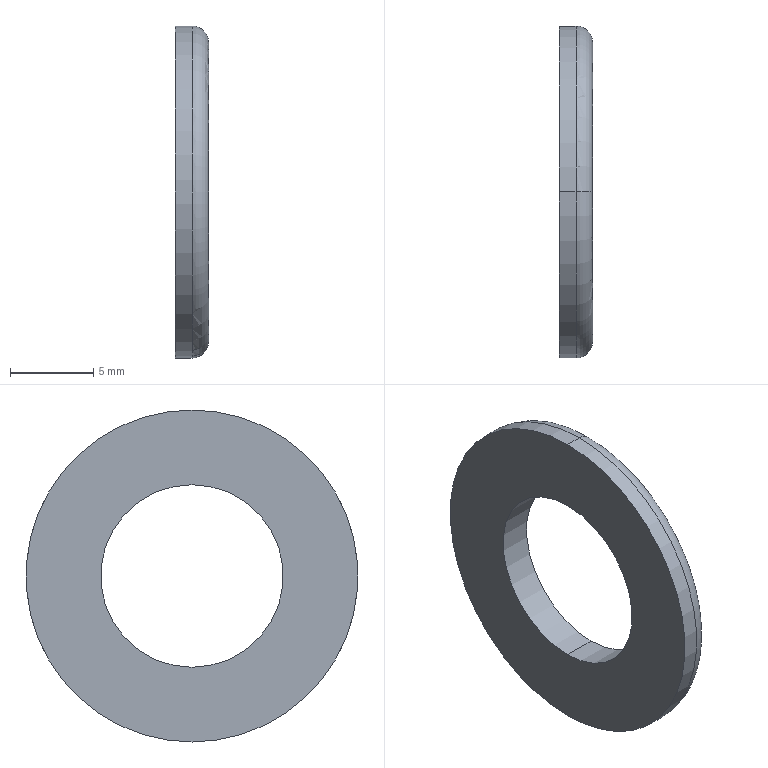Part | NX | features BREP 1 | 1 solid | 8 faces | box 2 x 20 x 20 mm | volume 425.07 mm3 | cylinder 4 | torus 2 | plane 2 | commonest cylinder face diameters 11 x2 20 x2
STEP:
#1=CARTESIAN_POINT('',(156.,0.,10.));
#2=VERTEX_POINT('',#1);
#3=CARTESIAN_POINT('',(156.,0.,-10.));
#4=VERTEX_POINT('',#3);
#5=CARTESIAN_POINT('',(156.,0.,0.));
#6=DIRECTION('',(1.,0.,0.));
#7=DIRECTION('',(0.,0.,1.));
#8=AXIS2_PLACEMENT_3D('',#5,#6,#7);
#9=CIRCLE('',#8,10.);
#10=EDGE_CURVE('',#2,#4,#9,.T.);
#11=ORIENTED_EDGE('',*,*,#10,.F.);
#12=CARTESIAN_POINT('',(155.,0.,10.));
#13=VERTEX_POINT('',#12);
#14=CARTESIAN_POINT('',(155.,0.,10.));
#15=DIRECTION('',(1.,0.,0.));
#16=VECTOR('',#15,1000.);
#17=LINE('',#14,#16);
#18=EDGE_CURVE('',#13,#2,#17,.T.);
#19=ORIENTED_EDGE('',*,*,#18,.F.);
#20=CARTESIAN_POINT('',(155.,0.,-10.));
#21=VERTEX_POINT('',#20);
#22=CARTESIAN_POINT('',(155.,0.,0.));
#23=DIRECTION('',(-1.,0.,0.));
#24=DIRECTION('',(0.,0.,-1.));
#25=AXIS2_PLACEMENT_3D('',#22,#23,#24);
#26=CIRCLE('',#25,10.);
#27=EDGE_CURVE('',#21,#13,#26,.T.);
#28=ORIENTED_EDGE('',*,*,#27,.F.);
#29=CARTESIAN_POINT('',(155.,0.,-10.));
#30=DIRECTION('',(1.,0.,0.));
#31=VECTOR('',#30,1000.);
#32=LINE('',#29,#31);
#33=EDGE_CURVE('',#21,#4,#32,.T.);
#34=ORIENTED_EDGE('',*,*,#33,.T.);
#35=EDGE_LOOP('',(#11,#19,#28,#34));
#36=FACE_BOUND('',#35,.T.);
#37=CARTESIAN_POINT('',(157.,0.,0.));
#38=DIRECTION('',(-1.,0.,0.));
#39=DIRECTION('',(0.,0.,-1.));
#40=AXIS2_PLACEMENT_3D('',#37,#38,#39);
#41=CYLINDRICAL_SURFACE('',#40,10.);
#42=ADVANCED_FACE('',(#36),#41,.T.);
#43=ORIENTED_EDGE('',*,*,#33,.F.);
#44=CARTESIAN_POINT('',(155.,0.,0.));
#45=DIRECTION('',(-1.,0.,0.));
#46=DIRECTION('',(0.,0.,1.));
#47=AXIS2_PLACEMENT_3D('',#44,#45,#46);
#48=CIRCLE('',#47,10.);
#49=EDGE_CURVE('',#13,#21,#48,.T.);
#50=ORIENTED_EDGE('',*,*,#49,.F.);
#51=ORIENTED_EDGE('',*,*,#18,.T.);
#52=CARTESIAN_POINT('',(156.,0.,0.));
#53=DIRECTION('',(1.,0.,0.));
#54=DIRECTION('',(0.,0.,-1.));
#55=AXIS2_PLACEMENT_3D('',#52,#53,#54);
#56=CIRCLE('',#55,10.);
#57=EDGE_CURVE('',#4,#2,#56,.T.);
#58=ORIENTED_EDGE('',*,*,#57,.F.);
#59=EDGE_LOOP('',(#43,#50,#51,#58));
#60=FACE_BOUND('',#59,.T.);
#61=CARTESIAN_POINT('',(157.,0.,0.));
#62=DIRECTION('',(-1.,0.,0.));
#63=DIRECTION('',(0.,0.,-1.));
#64=AXIS2_PLACEMENT_3D('',#61,#62,#63);
#65=CYLINDRICAL_SURFACE('',#64,10.);
#66=ADVANCED_FACE('',(#60),#65,.T.);
#67=CARTESIAN_POINT('',(157.,0.,9.));
#68=VERTEX_POINT('',#67);
#69=CARTESIAN_POINT('',(156.,0.,9.));
#70=DIRECTION('',(0.,-1.,0.));
#71=DIRECTION('',(1.,0.,0.));
#72=AXIS2_PLACEMENT_3D('',#69,#70,#71);
#73=CIRCLE('',#72,1.);
#74=EDGE_CURVE('',#68,#2,#73,.T.);
#75=ORIENTED_EDGE('',*,*,#74,.F.);
#76=CARTESIAN_POINT('',(157.,0.,-9.));
#77=VERTEX_POINT('',#76);
#78=CARTESIAN_POINT('',(157.,0.,0.));
#79=DIRECTION('',(1.,0.,0.));
#80=DIRECTION('',(0.,0.,-1.));
#81=AXIS2_PLACEMENT_3D('',#78,#79,#80);
#82=CIRCLE('',#81,9.);
#83=EDGE_CURVE('',#77,#68,#82,.T.);
#84=ORIENTED_EDGE('',*,*,#83,.F.);
#85=CARTESIAN_POINT('',(156.,0.,-9.));
#86=DIRECTION('',(0.,1.,0.));
#87=DIRECTION('',(1.,0.,0.));
#88=AXIS2_PLACEMENT_3D('',#85,#86,#87);
#89=CIRCLE('',#88,1.);
#90=EDGE_CURVE('',#77,#4,#89,.T.);
#91=ORIENTED_EDGE('',*,*,#90,.T.);
#92=ORIENTED_EDGE('',*,*,#57,.T.);
#93=EDGE_LOOP('',(#75,#84,#91,#92));
#94=FACE_BOUND('',#93,.T.);
#95=CARTESIAN_POINT('',(156.,0.,0.));
#96=DIRECTION('',(1.,0.,0.));
#97=DIRECTION('',(0.,0.,1.));
#98=AXIS2_PLACEMENT_3D('',#95,#96,#97);
#99=TOROIDAL_SURFACE('',#98,9.,1.);
#100=ADVANCED_FACE('',(#94),#99,.T.);
#101=ORIENTED_EDGE('',*,*,#10,.T.);
#102=ORIENTED_EDGE('',*,*,#90,.F.);
#103=CARTESIAN_POINT('',(157.,0.,0.));
#104=DIRECTION('',(1.,0.,0.));
#105=DIRECTION('',(0.,0.,1.));
#106=AXIS2_PLACEMENT_3D('',#103,#104,#105);
#107=CIRCLE('',#106,9.);
#108=EDGE_CURVE('',#68,#77,#107,.T.);
#109=ORIENTED_EDGE('',*,*,#108,.F.);
#110=ORIENTED_EDGE('',*,*,#74,.T.);
#111=EDGE_LOOP('',(#101,#102,#109,#110));
#112=FACE_BOUND('',#111,.T.);
#113=CARTESIAN_POINT('',(156.,0.,0.));
#114=DIRECTION('',(1.,0.,0.));
#115=DIRECTION('',(0.,0.,1.));
#116=AXIS2_PLACEMENT_3D('',#113,#114,#115);
#117=TOROIDAL_SURFACE('',#116,9.,1.);
#118=ADVANCED_FACE('',(#112),#117,.T.);
#119=ORIENTED_EDGE('',*,*,#108,.T.);
#120=ORIENTED_EDGE('',*,*,#83,.T.);
#121=EDGE_LOOP('',(#119,#120));
#122=FACE_BOUND('',#121,.T.);
#123=CARTESIAN_POINT('',(157.,0.,5.5));
#124=VERTEX_POINT('',#123);
#125=CARTESIAN_POINT('',(157.,0.,-5.5));
#126=VERTEX_POINT('',#125);
#127=CARTESIAN_POINT('',(157.,0.,0.));
#128=DIRECTION('',(-1.,0.,0.));
#129=DIRECTION('',(0.,0.,1.));
#130=AXIS2_PLACEMENT_3D('',#127,#128,#129);
#131=CIRCLE('',#130,5.5);
#132=EDGE_CURVE('',#124,#126,#131,.T.);
#133=ORIENTED_EDGE('',*,*,#132,.T.);
#134=CARTESIAN_POINT('',(157.,0.,0.));
#135=DIRECTION('',(-1.,0.,0.));
#136=DIRECTION('',(0.,0.,-1.));
#137=AXIS2_PLACEMENT_3D('',#134,#135,#136);
#138=CIRCLE('',#137,5.5);
#139=EDGE_CURVE('',#126,#124,#138,.T.);
#140=ORIENTED_EDGE('',*,*,#139,.T.);
#141=EDGE_LOOP('',(#133,#140));
#142=FACE_BOUND('',#141,.T.);
#143=CARTESIAN_POINT('',(157.,0.,0.));
#144=DIRECTION('',(1.,0.,0.));
#145=DIRECTION('',(0.,0.,1.));
#146=AXIS2_PLACEMENT_3D('',#143,#144,#145);
#147=PLANE('',#146);
#148=ADVANCED_FACE('',(#122,#142),#147,.T.);
#149=CARTESIAN_POINT('',(155.,0.,-5.5));
#150=VERTEX_POINT('',#149);
#151=CARTESIAN_POINT('',(155.,0.,-5.5));
#152=DIRECTION('',(1.,0.,0.));
#153=VECTOR('',#152,1000.);
#154=LINE('',#151,#153);
#155=EDGE_CURVE('',#126,#150,#154,.F.);
#156=ORIENTED_EDGE('',*,*,#155,.T.);
#157=CARTESIAN_POINT('',(155.,0.,5.5));
#158=VERTEX_POINT('',#157);
#159=CARTESIAN_POINT('',(155.,0.,0.));
#160=DIRECTION('',(1.,0.,0.));
#161=DIRECTION('',(0.,0.,1.));
#162=AXIS2_PLACEMENT_3D('',#159,#160,#161);
#163=CIRCLE('',#162,5.5);
#164=EDGE_CURVE('',#158,#150,#163,.T.);
#165=ORIENTED_EDGE('',*,*,#164,.F.);
#166=CARTESIAN_POINT('',(155.,0.,5.5));
#167=DIRECTION('',(1.,0.,0.));
#168=VECTOR('',#167,1000.);
#169=LINE('',#166,#168);
#170=EDGE_CURVE('',#124,#158,#169,.F.);
#171=ORIENTED_EDGE('',*,*,#170,.F.);
#172=ORIENTED_EDGE('',*,*,#139,.F.);
#173=EDGE_LOOP('',(#156,#165,#171,#172));
#174=FACE_BOUND('',#173,.T.);
#175=CARTESIAN_POINT('',(157.,0.,0.));
#176=DIRECTION('',(-1.,0.,0.));
#177=DIRECTION('',(0.,0.,-1.));
#178=AXIS2_PLACEMENT_3D('',#175,#176,#177);
#179=CYLINDRICAL_SURFACE('',#178,5.5);
#180=ADVANCED_FACE('',(#174),#179,.F.);
#181=ORIENTED_EDGE('',*,*,#132,.F.);
#182=ORIENTED_EDGE('',*,*,#170,.T.);
#183=CARTESIAN_POINT('',(155.,0.,0.));
#184=DIRECTION('',(1.,0.,0.));
#185=DIRECTION('',(0.,0.,-1.));
#186=AXIS2_PLACEMENT_3D('',#183,#184,#185);
#187=CIRCLE('',#186,5.5);
#188=EDGE_CURVE('',#150,#158,#187,.T.);
#189=ORIENTED_EDGE('',*,*,#188,.F.);
#190=ORIENTED_EDGE('',*,*,#155,.F.);
#191=EDGE_LOOP('',(#181,#182,#189,#190));
#192=FACE_BOUND('',#191,.T.);
#193=CARTESIAN_POINT('',(157.,0.,0.));
#194=DIRECTION('',(-1.,0.,0.));
#195=DIRECTION('',(0.,0.,-1.));
#196=AXIS2_PLACEMENT_3D('',#193,#194,#195);
#197=CYLINDRICAL_SURFACE('',#196,5.5);
#198=ADVANCED_FACE('',(#192),#197,.F.);
#199=ORIENTED_EDGE('',*,*,#49,.T.);
#200=ORIENTED_EDGE('',*,*,#27,.T.);
#201=EDGE_LOOP('',(#199,#200));
#202=FACE_BOUND('',#201,.T.);
#203=ORIENTED_EDGE('',*,*,#188,.T.);
#204=ORIENTED_EDGE('',*,*,#164,.T.);
#205=EDGE_LOOP('',(#203,#204));
#206=FACE_BOUND('',#205,.T.);
#207=CARTESIAN_POINT('',(155.,0.,0.));
#208=DIRECTION('',(1.,0.,0.));
#209=DIRECTION('',(0.,0.,1.));
#210=AXIS2_PLACEMENT_3D('',#207,#208,#209);
#211=PLANE('',#210);
#212=ADVANCED_FACE('',(#202,#206),#211,.F.);
#213=CLOSED_SHELL('',(#42,#66,#100,#118,#148,#180,#198,#212));
#214=MANIFOLD_SOLID_BREP('',#213);
#215=(LENGTH_UNIT()NAMED_UNIT(*)SI_UNIT(.MILLI.,.METRE.));
#216=UNCERTAINTY_MEASURE_WITH_UNIT(LENGTH_MEASURE(0.00001),#215,'','');
#217=(NAMED_UNIT(*)PLANE_ANGLE_UNIT()SI_UNIT($,.RADIAN.));
#218=(NAMED_UNIT(*)SI_UNIT($,.STERADIAN.)SOLID_ANGLE_UNIT());
#219=(GEOMETRIC_REPRESENTATION_CONTEXT(3)GLOBAL_UNCERTAINTY_ASSIGNED_CONTEXT((#216))GLOBAL_UNIT_ASSIGNED_CONTEXT((#215,#217,#218))REPRESENTATION_CONTEXT('',''));
#220=ADVANCED_BREP_SHAPE_REPRESENTATION('',(#214),#219);